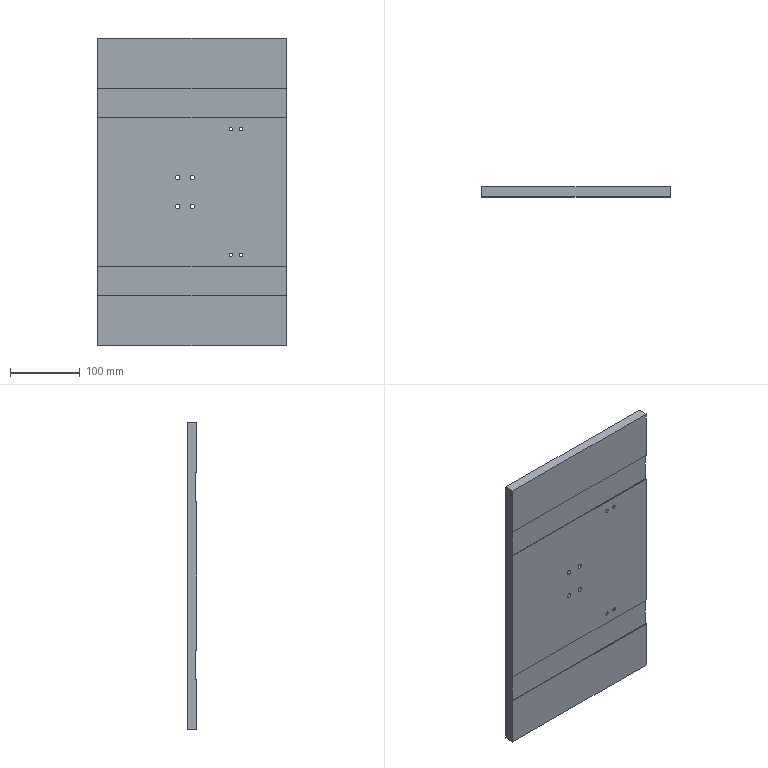Part | SolidWorks | features ICE 3, 3DProfileFeature 1, Extrusion 1, HoleWzd 1 | 1 solid | 47 faces | box 270 x 14 x 440 mm | volume 1620625 mm3 | cylinder 24 | plane 23 | commonest cylinder face diameters 5 x8 6.6 x8 11 x8
STEP:
#1=CARTESIAN_POINT('',(70.,0.,-92.5));
#2=VERTEX_POINT('',#1);
#3=CARTESIAN_POINT('',(70.,0.,-87.5));
#4=VERTEX_POINT('',#3);
#5=CARTESIAN_POINT('',(70.,0.,-90.));
#6=DIRECTION('',(0.,1.,0.));
#7=DIRECTION('',(0.,0.,-1.));
#8=AXIS2_PLACEMENT_3D('',#5,#6,#7);
#9=CIRCLE('',#8,2.5);
#10=EDGE_CURVE('',#2,#4,#9,.T.);
#11=ORIENTED_EDGE('',*,*,#10,.F.);
#12=CARTESIAN_POINT('',(70.,14.,-92.5));
#13=VERTEX_POINT('',#12);
#14=CARTESIAN_POINT('',(70.,-0.001,-92.5));
#15=DIRECTION('',(0.,1.,0.));
#16=VECTOR('',#15,1000.);
#17=LINE('',#14,#16);
#18=EDGE_CURVE('',#2,#13,#17,.T.);
#19=ORIENTED_EDGE('',*,*,#18,.T.);
#20=CARTESIAN_POINT('',(67.5,14.,-90.));
#21=VERTEX_POINT('',#20);
#22=CARTESIAN_POINT('',(70.,14.,-90.));
#23=DIRECTION('',(0.,1.,0.));
#24=DIRECTION('',(0.,0.,1.));
#25=AXIS2_PLACEMENT_3D('',#22,#23,#24);
#26=CIRCLE('',#25,2.5);
#27=EDGE_CURVE('',#13,#21,#26,.T.);
#28=ORIENTED_EDGE('',*,*,#27,.T.);
#29=CARTESIAN_POINT('',(67.5,12.5,-90.));
#30=VERTEX_POINT('',#29);
#31=CARTESIAN_POINT('',(67.5,-0.001,-90.));
#32=DIRECTION('',(0.,-1.,0.));
#33=VECTOR('',#32,1000.);
#34=LINE('',#31,#33);
#35=EDGE_CURVE('',#21,#30,#34,.T.);
#36=ORIENTED_EDGE('',*,*,#35,.T.);
#37=CARTESIAN_POINT('',(70.,12.5,-87.5));
#38=VERTEX_POINT('',#37);
#39=CARTESIAN_POINT('',(70.,12.5,-90.));
#40=DIRECTION('',(0.,-1.,0.));
#41=DIRECTION('',(0.,0.,1.));
#42=AXIS2_PLACEMENT_3D('',#39,#40,#41);
#43=CIRCLE('',#42,2.5);
#44=EDGE_CURVE('',#38,#30,#43,.T.);
#45=ORIENTED_EDGE('',*,*,#44,.F.);
#46=CARTESIAN_POINT('',(70.,-0.001,-87.5));
#47=DIRECTION('',(0.,1.,0.));
#48=VECTOR('',#47,1000.);
#49=LINE('',#46,#48);
#50=EDGE_CURVE('',#4,#38,#49,.T.);
#51=ORIENTED_EDGE('',*,*,#50,.F.);
#52=EDGE_LOOP('',(#11,#19,#28,#36,#45,#51));
#53=FACE_OUTER_BOUND('',#52,.T.);
#54=CARTESIAN_POINT('',(70.,-0.001,-90.));
#55=DIRECTION('',(0.,1.,0.));
#56=DIRECTION('',(0.,0.,1.));
#57=AXIS2_PLACEMENT_3D('',#54,#55,#56);
#58=CYLINDRICAL_SURFACE('',#57,2.5);
#59=ADVANCED_FACE('',(#53),#58,.F.);
#60=CARTESIAN_POINT('',(55.5,0.,87.5));
#61=VERTEX_POINT('',#60);
#62=CARTESIAN_POINT('',(55.5,0.,92.5));
#63=VERTEX_POINT('',#62);
#64=CARTESIAN_POINT('',(55.5,0.,90.));
#65=DIRECTION('',(0.,1.,0.));
#66=DIRECTION('',(0.,0.,-1.));
#67=AXIS2_PLACEMENT_3D('',#64,#65,#66);
#68=CIRCLE('',#67,2.5);
#69=EDGE_CURVE('',#61,#63,#68,.T.);
#70=ORIENTED_EDGE('',*,*,#69,.F.);
#71=CARTESIAN_POINT('',(55.5,12.5,87.5));
#72=VERTEX_POINT('',#71);
#73=CARTESIAN_POINT('',(55.5,-0.001,87.5));
#74=DIRECTION('',(0.,1.,0.));
#75=VECTOR('',#74,1000.);
#76=LINE('',#73,#75);
#77=EDGE_CURVE('',#61,#72,#76,.T.);
#78=ORIENTED_EDGE('',*,*,#77,.T.);
#79=CARTESIAN_POINT('',(55.5,14.,87.5));
#80=VERTEX_POINT('',#79);
#81=CARTESIAN_POINT('',(55.5,-0.001,87.5));
#82=DIRECTION('',(0.,1.,0.));
#83=VECTOR('',#82,1000.);
#84=LINE('',#81,#83);
#85=EDGE_CURVE('',#72,#80,#84,.T.);
#86=ORIENTED_EDGE('',*,*,#85,.T.);
#87=CARTESIAN_POINT('',(55.5,14.,92.5));
#88=VERTEX_POINT('',#87);
#89=CARTESIAN_POINT('',(55.5,14.,90.));
#90=DIRECTION('',(0.,1.,0.));
#91=DIRECTION('',(0.,0.,1.));
#92=AXIS2_PLACEMENT_3D('',#89,#90,#91);
#93=CIRCLE('',#92,2.5);
#94=EDGE_CURVE('',#80,#88,#93,.T.);
#95=ORIENTED_EDGE('',*,*,#94,.T.);
#96=CARTESIAN_POINT('',(55.5,-0.001,92.5));
#97=DIRECTION('',(0.,1.,0.));
#98=VECTOR('',#97,1000.);
#99=LINE('',#96,#98);
#100=EDGE_CURVE('',#63,#88,#99,.T.);
#101=ORIENTED_EDGE('',*,*,#100,.F.);
#102=EDGE_LOOP('',(#70,#78,#86,#95,#101));
#103=FACE_OUTER_BOUND('',#102,.T.);
#104=CARTESIAN_POINT('',(55.5,-0.001,90.));
#105=DIRECTION('',(0.,1.,0.));
#106=DIRECTION('',(0.,0.,1.));
#107=AXIS2_PLACEMENT_3D('',#104,#105,#106);
#108=CYLINDRICAL_SURFACE('',#107,2.5);
#109=ADVANCED_FACE('',(#103),#108,.F.);
#110=CARTESIAN_POINT('',(70.,0.,87.5));
#111=VERTEX_POINT('',#110);
#112=CARTESIAN_POINT('',(70.,0.,92.5));
#113=VERTEX_POINT('',#112);
#114=CARTESIAN_POINT('',(70.,0.,90.));
#115=DIRECTION('',(0.,1.,0.));
#116=DIRECTION('',(0.,0.,-1.));
#117=AXIS2_PLACEMENT_3D('',#114,#115,#116);
#118=CIRCLE('',#117,2.5);
#119=EDGE_CURVE('',#111,#113,#118,.T.);
#120=ORIENTED_EDGE('',*,*,#119,.F.);
#121=CARTESIAN_POINT('',(70.,12.5,87.5));
#122=VERTEX_POINT('',#121);
#123=CARTESIAN_POINT('',(70.,-0.001,87.5));
#124=DIRECTION('',(0.,1.,0.));
#125=VECTOR('',#124,1000.);
#126=LINE('',#123,#125);
#127=EDGE_CURVE('',#111,#122,#126,.T.);
#128=ORIENTED_EDGE('',*,*,#127,.T.);
#129=CARTESIAN_POINT('',(67.5,12.5,90.));
#130=VERTEX_POINT('',#129);
#131=CARTESIAN_POINT('',(70.,12.5,90.));
#132=DIRECTION('',(0.,-1.,0.));
#133=DIRECTION('',(0.,0.,1.));
#134=AXIS2_PLACEMENT_3D('',#131,#132,#133);
#135=CIRCLE('',#134,2.5);
#136=EDGE_CURVE('',#130,#122,#135,.T.);
#137=ORIENTED_EDGE('',*,*,#136,.F.);
#138=CARTESIAN_POINT('',(67.5,14.,90.));
#139=VERTEX_POINT('',#138);
#140=CARTESIAN_POINT('',(67.5,-0.001,90.));
#141=DIRECTION('',(0.,1.,0.));
#142=VECTOR('',#141,1000.);
#143=LINE('',#140,#142);
#144=EDGE_CURVE('',#130,#139,#143,.T.);
#145=ORIENTED_EDGE('',*,*,#144,.T.);
#146=CARTESIAN_POINT('',(70.,14.,92.5));
#147=VERTEX_POINT('',#146);
#148=CARTESIAN_POINT('',(70.,14.,90.));
#149=DIRECTION('',(0.,1.,0.));
#150=DIRECTION('',(0.,0.,1.));
#151=AXIS2_PLACEMENT_3D('',#148,#149,#150);
#152=CIRCLE('',#151,2.5);
#153=EDGE_CURVE('',#139,#147,#152,.T.);
#154=ORIENTED_EDGE('',*,*,#153,.T.);
#155=CARTESIAN_POINT('',(70.,-0.001,92.5));
#156=DIRECTION('',(0.,1.,0.));
#157=VECTOR('',#156,1000.);
#158=LINE('',#155,#157);
#159=EDGE_CURVE('',#113,#147,#158,.T.);
#160=ORIENTED_EDGE('',*,*,#159,.F.);
#161=EDGE_LOOP('',(#120,#128,#137,#145,#154,#160));
#162=FACE_OUTER_BOUND('',#161,.T.);
#163=CARTESIAN_POINT('',(70.,-0.001,90.));
#164=DIRECTION('',(0.,1.,0.));
#165=DIRECTION('',(0.,0.,1.));
#166=AXIS2_PLACEMENT_3D('',#163,#164,#165);
#167=CYLINDRICAL_SURFACE('',#166,2.5);
#168=ADVANCED_FACE('',(#162),#167,.F.);
#169=CARTESIAN_POINT('',(55.5,0.,-92.5));
#170=VERTEX_POINT('',#169);
#171=CARTESIAN_POINT('',(55.5,0.,-87.5));
#172=VERTEX_POINT('',#171);
#173=CARTESIAN_POINT('',(55.5,0.,-90.));
#174=DIRECTION('',(0.,1.,0.));
#175=DIRECTION('',(0.,0.,-1.));
#176=AXIS2_PLACEMENT_3D('',#173,#174,#175);
#177=CIRCLE('',#176,2.5);
#178=EDGE_CURVE('',#170,#172,#177,.T.);
#179=ORIENTED_EDGE('',*,*,#178,.F.);
#180=CARTESIAN_POINT('',(55.5,14.,-92.5));
#181=VERTEX_POINT('',#180);
#182=CARTESIAN_POINT('',(55.5,-0.001,-92.5));
#183=DIRECTION('',(0.,1.,0.));
#184=VECTOR('',#183,1000.);
#185=LINE('',#182,#184);
#186=EDGE_CURVE('',#170,#181,#185,.T.);
#187=ORIENTED_EDGE('',*,*,#186,.T.);
#188=CARTESIAN_POINT('',(55.5,14.,-87.5));
#189=VERTEX_POINT('',#188);
#190=CARTESIAN_POINT('',(55.5,14.,-90.));
#191=DIRECTION('',(0.,1.,0.));
#192=DIRECTION('',(0.,0.,1.));
#193=AXIS2_PLACEMENT_3D('',#190,#191,#192);
#194=CIRCLE('',#193,2.5);
#195=EDGE_CURVE('',#181,#189,#194,.T.);
#196=ORIENTED_EDGE('',*,*,#195,.T.);
#197=CARTESIAN_POINT('',(55.5,12.5,-87.5));
#198=VERTEX_POINT('',#197);
#199=CARTESIAN_POINT('',(55.5,-0.001,-87.5));
#200=DIRECTION('',(0.,-1.,0.));
#201=VECTOR('',#200,1000.);
#202=LINE('',#199,#201);
#203=EDGE_CURVE('',#189,#198,#202,.T.);
#204=ORIENTED_EDGE('',*,*,#203,.T.);
#205=CARTESIAN_POINT('',(55.5,-0.001,-87.5));
#206=DIRECTION('',(0.,1.,0.));
#207=VECTOR('',#206,1000.);
#208=LINE('',#205,#207);
#209=EDGE_CURVE('',#172,#198,#208,.T.);
#210=ORIENTED_EDGE('',*,*,#209,.F.);
#211=EDGE_LOOP('',(#179,#187,#196,#204,#210));
#212=FACE_OUTER_BOUND('',#211,.T.);
#213=CARTESIAN_POINT('',(55.5,-0.001,-90.));
#214=DIRECTION('',(0.,1.,0.));
#215=DIRECTION('',(0.,0.,1.));
#216=AXIS2_PLACEMENT_3D('',#213,#214,#215);
#217=CYLINDRICAL_SURFACE('',#216,2.5);
#218=ADVANCED_FACE('',(#212),#217,.F.);
#219=CARTESIAN_POINT('',(-20.55,7.2,15.));
#220=VERTEX_POINT('',#219);
#221=CARTESIAN_POINT('',(-20.55,7.2,26.));
#222=VERTEX_POINT('',#221);
#223=CARTESIAN_POINT('',(-20.55,7.2,20.5));
#224=DIRECTION('',(0.,1.,0.));
#225=DIRECTION('',(0.,0.,1.));
#226=AXIS2_PLACEMENT_3D('',#223,#224,#225);
#227=CIRCLE('',#226,5.5);
#228=EDGE_CURVE('',#220,#222,#227,.T.);
#229=ORIENTED_EDGE('',*,*,#228,.F.);
#230=CARTESIAN_POINT('',(-20.55,14.,15.));
#231=VERTEX_POINT('',#230);
#232=CARTESIAN_POINT('',(-20.55,14.,15.));
#233=DIRECTION('',(0.,1.,0.));
#234=VECTOR('',#233,1000.);
#235=LINE('',#232,#234);
#236=EDGE_CURVE('',#220,#231,#235,.T.);
#237=ORIENTED_EDGE('',*,*,#236,.T.);
#238=CARTESIAN_POINT('',(-20.55,14.,26.));
#239=VERTEX_POINT('',#238);
#240=CARTESIAN_POINT('',(-20.55,14.,20.5));
#241=DIRECTION('',(0.,1.,0.));
#242=DIRECTION('',(0.,0.,1.));
#243=AXIS2_PLACEMENT_3D('',#240,#241,#242);
#244=CIRCLE('',#243,5.5);
#245=EDGE_CURVE('',#231,#239,#244,.T.);
#246=ORIENTED_EDGE('',*,*,#245,.T.);
#247=CARTESIAN_POINT('',(-20.55,14.,26.));
#248=DIRECTION('',(0.,1.,0.));
#249=VECTOR('',#248,1000.);
#250=LINE('',#247,#249);
#251=EDGE_CURVE('',#222,#239,#250,.T.);
#252=ORIENTED_EDGE('',*,*,#251,.F.);
#253=EDGE_LOOP('',(#229,#237,#246,#252));
#254=FACE_OUTER_BOUND('',#253,.T.);
#255=CARTESIAN_POINT('',(-20.55,14.,20.5));
#256=DIRECTION('',(0.,1.,0.));
#257=DIRECTION('',(0.,0.,1.));
#258=AXIS2_PLACEMENT_3D('',#255,#256,#257);
#259=CYLINDRICAL_SURFACE('',#258,5.5);
#260=ADVANCED_FACE('',(#254),#259,.F.);
#261=CARTESIAN_POINT('',(-20.55,0.,23.8));
#262=VERTEX_POINT('',#261);
#263=CARTESIAN_POINT('',(-20.55,0.,17.2));
#264=VERTEX_POINT('',#263);
#265=CARTESIAN_POINT('',(-20.55,0.,20.5));
#266=DIRECTION('',(0.,-1.,0.));
#267=DIRECTION('',(0.,0.,-1.));
#268=AXIS2_PLACEMENT_3D('',#265,#266,#267);
#269=CIRCLE('',#268,3.3);
#270=EDGE_CURVE('',#262,#264,#269,.T.);
#271=ORIENTED_EDGE('',*,*,#270,.T.);
#272=CARTESIAN_POINT('',(-20.55,7.2,17.2));
#273=VERTEX_POINT('',#272);
#274=CARTESIAN_POINT('',(-20.55,14.,17.2));
#275=DIRECTION('',(0.,1.,0.));
#276=VECTOR('',#275,1000.);
#277=LINE('',#274,#276);
#278=EDGE_CURVE('',#264,#273,#277,.T.);
#279=ORIENTED_EDGE('',*,*,#278,.T.);
#280=CARTESIAN_POINT('',(-20.55,7.2,23.8));
#281=VERTEX_POINT('',#280);
#282=CARTESIAN_POINT('',(-20.55,7.2,20.5));
#283=DIRECTION('',(0.,1.,0.));
#284=DIRECTION('',(0.,0.,1.));
#285=AXIS2_PLACEMENT_3D('',#282,#283,#284);
#286=CIRCLE('',#285,3.3);
#287=EDGE_CURVE('',#273,#281,#286,.T.);
#288=ORIENTED_EDGE('',*,*,#287,.T.);
#289=CARTESIAN_POINT('',(-20.55,14.,23.8));
#290=DIRECTION('',(0.,1.,0.));
#291=VECTOR('',#290,1000.);
#292=LINE('',#289,#291);
#293=EDGE_CURVE('',#262,#281,#292,.T.);
#294=ORIENTED_EDGE('',*,*,#293,.F.);
#295=EDGE_LOOP('',(#271,#279,#288,#294));
#296=FACE_OUTER_BOUND('',#295,.T.);
#297=CARTESIAN_POINT('',(-20.55,14.,20.5));
#298=DIRECTION('',(0.,1.,0.));
#299=DIRECTION('',(0.,0.,1.));
#300=AXIS2_PLACEMENT_3D('',#297,#298,#299);
#301=CYLINDRICAL_SURFACE('',#300,3.3);
#302=ADVANCED_FACE('',(#296),#301,.F.);
#303=CARTESIAN_POINT('',(-20.55,7.2,-26.));
#304=VERTEX_POINT('',#303);
#305=CARTESIAN_POINT('',(-20.55,7.2,-15.));
#306=VERTEX_POINT('',#305);
#307=CARTESIAN_POINT('',(-20.55,7.2,-20.5));
#308=DIRECTION('',(0.,1.,0.));
#309=DIRECTION('',(0.,0.,1.));
#310=AXIS2_PLACEMENT_3D('',#307,#308,#309);
#311=CIRCLE('',#310,5.5);
#312=EDGE_CURVE('',#304,#306,#311,.T.);
#313=ORIENTED_EDGE('',*,*,#312,.F.);
#314=CARTESIAN_POINT('',(-20.55,14.,-26.));
#315=VERTEX_POINT('',#314);
#316=CARTESIAN_POINT('',(-20.55,14.,-26.));
#317=DIRECTION('',(0.,1.,0.));
#318=VECTOR('',#317,1000.);
#319=LINE('',#316,#318);
#320=EDGE_CURVE('',#304,#315,#319,.T.);
#321=ORIENTED_EDGE('',*,*,#320,.T.);
#322=CARTESIAN_POINT('',(-20.55,14.,-15.));
#323=VERTEX_POINT('',#322);
#324=CARTESIAN_POINT('',(-20.55,14.,-20.5));
#325=DIRECTION('',(0.,1.,0.));
#326=DIRECTION('',(0.,0.,1.));
#327=AXIS2_PLACEMENT_3D('',#324,#325,#326);
#328=CIRCLE('',#327,5.5);
#329=EDGE_CURVE('',#315,#323,#328,.T.);
#330=ORIENTED_EDGE('',*,*,#329,.T.);
#331=CARTESIAN_POINT('',(-20.55,14.,-15.));
#332=DIRECTION('',(0.,1.,0.));
#333=VECTOR('',#332,1000.);
#334=LINE('',#331,#333);
#335=EDGE_CURVE('',#306,#323,#334,.T.);
#336=ORIENTED_EDGE('',*,*,#335,.F.);
#337=EDGE_LOOP('',(#313,#321,#330,#336));
#338=FACE_OUTER_BOUND('',#337,.T.);
#339=CARTESIAN_POINT('',(-20.55,14.,-20.5));
#340=DIRECTION('',(0.,1.,0.));
#341=DIRECTION('',(0.,0.,1.));
#342=AXIS2_PLACEMENT_3D('',#339,#340,#341);
#343=CYLINDRICAL_SURFACE('',#342,5.5);
#344=ADVANCED_FACE('',(#338),#343,.F.);
#345=CARTESIAN_POINT('',(-20.55,0.,-17.2));
#346=VERTEX_POINT('',#345);
#347=CARTESIAN_POINT('',(-20.55,0.,-23.8));
#348=VERTEX_POINT('',#347);
#349=CARTESIAN_POINT('',(-20.55,0.,-20.5));
#350=DIRECTION('',(0.,-1.,0.));
#351=DIRECTION('',(0.,0.,-1.));
#352=AXIS2_PLACEMENT_3D('',#349,#350,#351);
#353=CIRCLE('',#352,3.3);
#354=EDGE_CURVE('',#346,#348,#353,.T.);
#355=ORIENTED_EDGE('',*,*,#354,.T.);
#356=CARTESIAN_POINT('',(-20.55,7.2,-23.8));
#357=VERTEX_POINT('',#356);
#358=CARTESIAN_POINT('',(-20.55,14.,-23.8));
#359=DIRECTION('',(0.,1.,0.));
#360=VECTOR('',#359,1000.);
#361=LINE('',#358,#360);
#362=EDGE_CURVE('',#348,#357,#361,.T.);
#363=ORIENTED_EDGE('',*,*,#362,.T.);
#364=CARTESIAN_POINT('',(-20.55,7.2,-17.2));
#365=VERTEX_POINT('',#364);
#366=CARTESIAN_POINT('',(-20.55,7.2,-20.5));
#367=DIRECTION('',(0.,1.,0.));
#368=DIRECTION('',(0.,0.,1.));
#369=AXIS2_PLACEMENT_3D('',#366,#367,#368);
#370=CIRCLE('',#369,3.3);
#371=EDGE_CURVE('',#357,#365,#370,.T.);
#372=ORIENTED_EDGE('',*,*,#371,.T.);
#373=CARTESIAN_POINT('',(-20.55,14.,-17.2));
#374=DIRECTION('',(0.,1.,0.));
#375=VECTOR('',#374,1000.);
#376=LINE('',#373,#375);
#377=EDGE_CURVE('',#346,#365,#376,.T.);
#378=ORIENTED_EDGE('',*,*,#377,.F.);
#379=EDGE_LOOP('',(#355,#363,#372,#378));
#380=FACE_OUTER_BOUND('',#379,.T.);
#381=CARTESIAN_POINT('',(-20.55,14.,-20.5));
#382=DIRECTION('',(0.,1.,0.));
#383=DIRECTION('',(0.,0.,1.));
#384=AXIS2_PLACEMENT_3D('',#381,#382,#383);
#385=CYLINDRICAL_SURFACE('',#384,3.3);
#386=ADVANCED_FACE('',(#380),#385,.F.);
#387=CARTESIAN_POINT('',(0.45,7.2,15.));
#388=VERTEX_POINT('',#387);
#389=CARTESIAN_POINT('',(0.45,7.2,26.));
#390=VERTEX_POINT('',#389);
#391=CARTESIAN_POINT('',(0.45,7.2,20.5));
#392=DIRECTION('',(0.,1.,0.));
#393=DIRECTION('',(0.,0.,1.));
#394=AXIS2_PLACEMENT_3D('',#391,#392,#393);
#395=CIRCLE('',#394,5.5);
#396=EDGE_CURVE('',#388,#390,#395,.T.);
#397=ORIENTED_EDGE('',*,*,#396,.F.);
#398=CARTESIAN_POINT('',(0.45,14.,15.));
#399=VERTEX_POINT('',#398);
#400=CARTESIAN_POINT('',(0.45,14.,15.));
#401=DIRECTION('',(0.,1.,0.));
#402=VECTOR('',#401,1000.);
#403=LINE('',#400,#402);
#404=EDGE_CURVE('',#388,#399,#403,.T.);
#405=ORIENTED_EDGE('',*,*,#404,.T.);
#406=CARTESIAN_POINT('',(0.45,14.,26.));
#407=VERTEX_POINT('',#406);
#408=CARTESIAN_POINT('',(0.45,14.,20.5));
#409=DIRECTION('',(0.,1.,0.));
#410=DIRECTION('',(0.,0.,1.));
#411=AXIS2_PLACEMENT_3D('',#408,#409,#410);
#412=CIRCLE('',#411,5.5);
#413=EDGE_CURVE('',#399,#407,#412,.T.);
#414=ORIENTED_EDGE('',*,*,#413,.T.);
#415=CARTESIAN_POINT('',(0.45,14.,26.));
#416=DIRECTION('',(0.,1.,0.));
#417=VECTOR('',#416,1000.);
#418=LINE('',#415,#417);
#419=EDGE_CURVE('',#390,#407,#418,.T.);
#420=ORIENTED_EDGE('',*,*,#419,.F.);
#421=EDGE_LOOP('',(#397,#405,#414,#420));
#422=FACE_OUTER_BOUND('',#421,.T.);
#423=CARTESIAN_POINT('',(0.45,14.,20.5));
#424=DIRECTION('',(0.,1.,0.));
#425=DIRECTION('',(0.,0.,1.));
#426=AXIS2_PLACEMENT_3D('',#423,#424,#425);
#427=CYLINDRICAL_SURFACE('',#426,5.5);
#428=ADVANCED_FACE('',(#422),#427,.F.);
#429=CARTESIAN_POINT('',(0.45,0.,23.8));
#430=VERTEX_POINT('',#429);
#431=CARTESIAN_POINT('',(0.45,0.,17.2));
#432=VERTEX_POINT('',#431);
#433=CARTESIAN_POINT('',(0.45,0.,20.5));
#434=DIRECTION('',(0.,-1.,0.));
#435=DIRECTION('',(0.,0.,-1.));
#436=AXIS2_PLACEMENT_3D('',#433,#434,#435);
#437=CIRCLE('',#436,3.3);
#438=EDGE_CURVE('',#430,#432,#437,.T.);
#439=ORIENTED_EDGE('',*,*,#438,.T.);
#440=CARTESIAN_POINT('',(0.45,7.2,17.2));
#441=VERTEX_POINT('',#440);
#442=CARTESIAN_POINT('',(0.45,14.,17.2));
#443=DIRECTION('',(0.,1.,0.));
#444=VECTOR('',#443,1000.);
#445=LINE('',#442,#444);
#446=EDGE_CURVE('',#432,#441,#445,.T.);
#447=ORIENTED_EDGE('',*,*,#446,.T.);
#448=CARTESIAN_POINT('',(0.45,7.2,23.8));
#449=VERTEX_POINT('',#448);
#450=CARTESIAN_POINT('',(0.45,7.2,20.5));
#451=DIRECTION('',(0.,1.,0.));
#452=DIRECTION('',(0.,0.,1.));
#453=AXIS2_PLACEMENT_3D('',#450,#451,#452);
#454=CIRCLE('',#453,3.3);
#455=EDGE_CURVE('',#441,#449,#454,.T.);
#456=ORIENTED_EDGE('',*,*,#455,.T.);
#457=CARTESIAN_POINT('',(0.45,14.,23.8));
#458=DIRECTION('',(0.,1.,0.));
#459=VECTOR('',#458,1000.);
#460=LINE('',#457,#459);
#461=EDGE_CURVE('',#430,#449,#460,.T.);
#462=ORIENTED_EDGE('',*,*,#461,.F.);
#463=EDGE_LOOP('',(#439,#447,#456,#462));
#464=FACE_OUTER_BOUND('',#463,.T.);
#465=CARTESIAN_POINT('',(0.45,14.,20.5));
#466=DIRECTION('',(0.,1.,0.));
#467=DIRECTION('',(0.,0.,1.));
#468=AXIS2_PLACEMENT_3D('',#465,#466,#467);
#469=CYLINDRICAL_SURFACE('',#468,3.3);
#470=ADVANCED_FACE('',(#464),#469,.F.);
#471=CARTESIAN_POINT('',(0.45,7.2,-26.));
#472=VERTEX_POINT('',#471);
#473=CARTESIAN_POINT('',(0.45,7.2,-15.));
#474=VERTEX_POINT('',#473);
#475=CARTESIAN_POINT('',(0.45,7.2,-20.5));
#476=DIRECTION('',(0.,1.,0.));
#477=DIRECTION('',(0.,0.,1.));
#478=AXIS2_PLACEMENT_3D('',#475,#476,#477);
#479=CIRCLE('',#478,5.5);
#480=EDGE_CURVE('',#472,#474,#479,.T.);
#481=ORIENTED_EDGE('',*,*,#480,.F.);
#482=CARTESIAN_POINT('',(0.45,14.,-26.));
#483=VERTEX_POINT('',#482);
#484=CARTESIAN_POINT('',(0.45,14.,-26.));
#485=DIRECTION('',(0.,1.,0.));
#486=VECTOR('',#485,1000.);
#487=LINE('',#484,#486);
#488=EDGE_CURVE('',#472,#483,#487,.T.);
#489=ORIENTED_EDGE('',*,*,#488,.T.);
#490=CARTESIAN_POINT('',(0.45,14.,-15.));
#491=VERTEX_POINT('',#490);
#492=CARTESIAN_POINT('',(0.45,14.,-20.5));
#493=DIRECTION('',(0.,1.,0.));
#494=DIRECTION('',(0.,0.,1.));
#495=AXIS2_PLACEMENT_3D('',#492,#493,#494);
#496=CIRCLE('',#495,5.5);
#497=EDGE_CURVE('',#483,#491,#496,.T.);
#498=ORIENTED_EDGE('',*,*,#497,.T.);
#499=CARTESIAN_POINT('',(0.45,14.,-15.));
#500=DIRECTION('',(0.,1.,0.));
#501=VECTOR('',#500,1000.);
#502=LINE('',#499,#501);
#503=EDGE_CURVE('',#474,#491,#502,.T.);
#504=ORIENTED_EDGE('',*,*,#503,.F.);
#505=EDGE_LOOP('',(#481,#489,#498,#504));
#506=FACE_OUTER_BOUND('',#505,.T.);
#507=CARTESIAN_POINT('',(0.45,14.,-20.5));
#508=DIRECTION('',(0.,1.,0.));
#509=DIRECTION('',(0.,0.,1.));
#510=AXIS2_PLACEMENT_3D('',#507,#508,#509);
#511=CYLINDRICAL_SURFACE('',#510,5.5);
#512=ADVANCED_FACE('',(#506),#511,.F.);
#513=CARTESIAN_POINT('',(0.45,0.,-17.2));
#514=VERTEX_POINT('',#513);
#515=CARTESIAN_POINT('',(0.45,0.,-23.8));
#516=VERTEX_POINT('',#515);
#517=CARTESIAN_POINT('',(0.45,0.,-20.5));
#518=DIRECTION('',(0.,-1.,0.));
#519=DIRECTION('',(0.,0.,-1.));
#520=AXIS2_PLACEMENT_3D('',#517,#518,#519);
#521=CIRCLE('',#520,3.3);
#522=EDGE_CURVE('',#514,#516,#521,.T.);
#523=ORIENTED_EDGE('',*,*,#522,.T.);
#524=CARTESIAN_POINT('',(0.45,7.2,-23.8));
#525=VERTEX_POINT('',#524);
#526=CARTESIAN_POINT('',(0.45,14.,-23.8));
#527=DIRECTION('',(0.,1.,0.));
#528=VECTOR('',#527,1000.);
#529=LINE('',#526,#528);
#530=EDGE_CURVE('',#516,#525,#529,.T.);
#531=ORIENTED_EDGE('',*,*,#530,.T.);
#532=CARTESIAN_POINT('',(0.45,7.2,-17.2));
#533=VERTEX_POINT('',#532);
#534=CARTESIAN_POINT('',(0.45,7.2,-20.5));
#535=DIRECTION('',(0.,1.,0.));
#536=DIRECTION('',(0.,0.,1.));
#537=AXIS2_PLACEMENT_3D('',#534,#535,#536);
#538=CIRCLE('',#537,3.3);
#539=EDGE_CURVE('',#525,#533,#538,.T.);
#540=ORIENTED_EDGE('',*,*,#539,.T.);
#541=CARTESIAN_POINT('',(0.45,14.,-17.2));
#542=DIRECTION('',(0.,1.,0.));
#543=VECTOR('',#542,1000.);
#544=LINE('',#541,#543);
#545=EDGE_CURVE('',#514,#533,#544,.T.);
#546=ORIENTED_EDGE('',*,*,#545,.F.);
#547=EDGE_LOOP('',(#523,#531,#540,#546));
#548=FACE_OUTER_BOUND('',#547,.T.);
#549=CARTESIAN_POINT('',(0.45,14.,-20.5));
#550=DIRECTION('',(0.,1.,0.));
#551=DIRECTION('',(0.,0.,1.));
#552=AXIS2_PLACEMENT_3D('',#549,#550,#551);
#553=CYLINDRICAL_SURFACE('',#552,3.3);
#554=ADVANCED_FACE('',(#548),#553,.F.);
#555=CARTESIAN_POINT('',(135.,0.,148.));
#556=VERTEX_POINT('',#555);
#557=CARTESIAN_POINT('',(-135.,0.,148.));
#558=VERTEX_POINT('',#557);
#559=CARTESIAN_POINT('',(-135.,0.,148.));
#560=DIRECTION('',(-1.,0.,0.));
#561=VECTOR('',#560,1000.);
#562=LINE('',#559,#561);
#563=EDGE_CURVE('',#556,#558,#562,.T.);
#564=ORIENTED_EDGE('',*,*,#563,.F.);
#565=CARTESIAN_POINT('',(135.,0.,220.));
#566=VERTEX_POINT('',#565);
#567=CARTESIAN_POINT('',(135.,0.,220.));
#568=DIRECTION('',(0.,0.,-1.));
#569=VECTOR('',#568,1000.);
#570=LINE('',#567,#569);
#571=EDGE_CURVE('',#566,#556,#570,.T.);
#572=ORIENTED_EDGE('',*,*,#571,.F.);
#573=CARTESIAN_POINT('',(-135.,0.,220.));
#574=VERTEX_POINT('',#573);
#575=CARTESIAN_POINT('',(-135.,0.,220.));
#576=DIRECTION('',(1.,0.,0.));
#577=VECTOR('',#576,1000.);
#578=LINE('',#575,#577);
#579=EDGE_CURVE('',#574,#566,#578,.T.);
#580=ORIENTED_EDGE('',*,*,#579,.F.);
#581=CARTESIAN_POINT('',(-135.,0.,220.));
#582=DIRECTION('',(0.,0.,1.));
#583=VECTOR('',#582,1000.);
#584=LINE('',#581,#583);
#585=EDGE_CURVE('',#558,#574,#584,.T.);
#586=ORIENTED_EDGE('',*,*,#585,.F.);
#587=EDGE_LOOP('',(#564,#572,#580,#586));
#588=FACE_OUTER_BOUND('',#587,.T.);
#589=CARTESIAN_POINT('',(0.,0.,0.));
#590=DIRECTION('',(0.,-1.,0.));
#591=DIRECTION('',(0.,0.,-1.));
#592=AXIS2_PLACEMENT_3D('',#589,#590,#591);
#593=PLANE('',#592);
#594=ADVANCED_FACE('',(#588),#593,.T.);
#595=CARTESIAN_POINT('',(70.,0.,-90.));
#596=DIRECTION('',(0.,1.,0.));
#597=DIRECTION('',(0.,0.,-1.));
#598=AXIS2_PLACEMENT_3D('',#595,#596,#597);
#599=CIRCLE('',#598,2.5);
#600=EDGE_CURVE('',#4,#2,#599,.T.);
#601=ORIENTED_EDGE('',*,*,#600,.T.);
#602=ORIENTED_EDGE('',*,*,#10,.T.);
#603=EDGE_LOOP('',(#601,#602));
#604=FACE_BOUND('',#603,.T.);
#605=CARTESIAN_POINT('',(55.5,0.,90.));
#606=DIRECTION('',(0.,1.,0.));
#607=DIRECTION('',(0.,0.,-1.));
#608=AXIS2_PLACEMENT_3D('',#605,#606,#607);
#609=CIRCLE('',#608,2.5);
#610=EDGE_CURVE('',#63,#61,#609,.T.);
#611=ORIENTED_EDGE('',*,*,#610,.T.);
#612=ORIENTED_EDGE('',*,*,#69,.T.);
#613=EDGE_LOOP('',(#611,#612));
#614=FACE_BOUND('',#613,.T.);
#615=CARTESIAN_POINT('',(70.,0.,90.));
#616=DIRECTION('',(0.,1.,0.));
#617=DIRECTION('',(0.,0.,-1.));
#618=AXIS2_PLACEMENT_3D('',#615,#616,#617);
#619=CIRCLE('',#618,2.5);
#620=EDGE_CURVE('',#113,#111,#619,.T.);
#621=ORIENTED_EDGE('',*,*,#620,.T.);
#622=ORIENTED_EDGE('',*,*,#119,.T.);
#623=EDGE_LOOP('',(#621,#622));
#624=FACE_BOUND('',#623,.T.);
#625=CARTESIAN_POINT('',(55.5,0.,-90.));
#626=DIRECTION('',(0.,1.,0.));
#627=DIRECTION('',(0.,0.,-1.));
#628=AXIS2_PLACEMENT_3D('',#625,#626,#627);
#629=CIRCLE('',#628,2.5);
#630=EDGE_CURVE('',#172,#170,#629,.T.);
#631=ORIENTED_EDGE('',*,*,#630,.T.);
#632=ORIENTED_EDGE('',*,*,#178,.T.);
#633=EDGE_LOOP('',(#631,#632));
#634=FACE_BOUND('',#633,.T.);
#635=ORIENTED_EDGE('',*,*,#270,.F.);
#636=CARTESIAN_POINT('',(-20.55,0.,20.5));
#637=DIRECTION('',(0.,-1.,0.));
#638=DIRECTION('',(0.,0.,-1.));
#639=AXIS2_PLACEMENT_3D('',#636,#637,#638);
#640=CIRCLE('',#639,3.3);
#641=EDGE_CURVE('',#264,#262,#640,.T.);
#642=ORIENTED_EDGE('',*,*,#641,.F.);
#643=EDGE_LOOP('',(#635,#642));
#644=FACE_BOUND('',#643,.T.);
#645=ORIENTED_EDGE('',*,*,#354,.F.);
#646=CARTESIAN_POINT('',(-20.55,0.,-20.5));
#647=DIRECTION('',(0.,-1.,0.));
#648=DIRECTION('',(0.,0.,-1.));
#649=AXIS2_PLACEMENT_3D('',#646,#647,#648);
#650=CIRCLE('',#649,3.3);
#651=EDGE_CURVE('',#348,#346,#650,.T.);
#652=ORIENTED_EDGE('',*,*,#651,.F.);
#653=EDGE_LOOP('',(#645,#652));
#654=FACE_BOUND('',#653,.T.);
#655=ORIENTED_EDGE('',*,*,#438,.F.);
#656=CARTESIAN_POINT('',(0.45,0.,20.5));
#657=DIRECTION('',(0.,-1.,0.));
#658=DIRECTION('',(0.,0.,-1.));
#659=AXIS2_PLACEMENT_3D('',#656,#657,#658);
#660=CIRCLE('',#659,3.3);
#661=EDGE_CURVE('',#432,#430,#660,.T.);
#662=ORIENTED_EDGE('',*,*,#661,.F.);
#663=EDGE_LOOP('',(#655,#662));
#664=FACE_BOUND('',#663,.T.);
#665=ORIENTED_EDGE('',*,*,#522,.F.);
#666=CARTESIAN_POINT('',(0.45,0.,-20.5));
#667=DIRECTION('',(0.,-1.,0.));
#668=DIRECTION('',(0.,0.,-1.));
#669=AXIS2_PLACEMENT_3D('',#666,#667,#668);
#670=CIRCLE('',#669,3.3);
#671=EDGE_CURVE('',#516,#514,#670,.T.);
#672=ORIENTED_EDGE('',*,*,#671,.F.);
#673=EDGE_LOOP('',(#665,#672));
#674=FACE_BOUND('',#673,.T.);
#675=CARTESIAN_POINT('',(-135.,0.,106.));
#676=VERTEX_POINT('',#675);
#677=CARTESIAN_POINT('',(135.,0.,106.));
#678=VERTEX_POINT('',#677);
#679=CARTESIAN_POINT('',(-135.,0.,106.));
#680=DIRECTION('',(1.,0.,0.));
#681=VECTOR('',#680,1000.);
#682=LINE('',#679,#681);
#683=EDGE_CURVE('',#676,#678,#682,.T.);
#684=ORIENTED_EDGE('',*,*,#683,.F.);
#685=CARTESIAN_POINT('',(-135.,0.,-106.));
#686=VERTEX_POINT('',#685);
#687=CARTESIAN_POINT('',(-135.,0.,220.));
#688=DIRECTION('',(0.,0.,1.));
#689=VECTOR('',#688,1000.);
#690=LINE('',#687,#689);
#691=EDGE_CURVE('',#686,#676,#690,.T.);
#692=ORIENTED_EDGE('',*,*,#691,.F.);
#693=CARTESIAN_POINT('',(135.,0.,-106.));
#694=VERTEX_POINT('',#693);
#695=CARTESIAN_POINT('',(-135.,0.,-106.));
#696=DIRECTION('',(-1.,0.,0.));
#697=VECTOR('',#696,1000.);
#698=LINE('',#695,#697);
#699=EDGE_CURVE('',#694,#686,#698,.T.);
#700=ORIENTED_EDGE('',*,*,#699,.F.);
#701=CARTESIAN_POINT('',(135.,0.,220.));
#702=DIRECTION('',(0.,0.,-1.));
#703=VECTOR('',#702,1000.);
#704=LINE('',#701,#703);
#705=EDGE_CURVE('',#678,#694,#704,.T.);
#706=ORIENTED_EDGE('',*,*,#705,.F.);
#707=EDGE_LOOP('',(#684,#692,#700,#706));
#708=FACE_OUTER_BOUND('',#707,.T.);
#709=CARTESIAN_POINT('',(0.,0.,0.));
#710=DIRECTION('',(0.,-1.,0.));
#711=DIRECTION('',(0.,0.,-1.));
#712=AXIS2_PLACEMENT_3D('',#709,#710,#711);
#713=PLANE('',#712);
#714=ADVANCED_FACE('',(#604,#614,#624,#634,#644,#654,#664,#674,#708),#713,.T.);
#715=ORIENTED_EDGE('',*,*,#571,.T.);
#716=CARTESIAN_POINT('',(135.,1.5,148.));
#717=VERTEX_POINT('',#716);
#718=CARTESIAN_POINT('',(135.,1.5,148.));
#719=DIRECTION('',(0.,-1.,0.));
#720=VECTOR('',#719,1000.);
#721=LINE('',#718,#720);
#722=EDGE_CURVE('',#717,#556,#721,.T.);
#723=ORIENTED_EDGE('',*,*,#722,.F.);
#724=CARTESIAN_POINT('',(135.,1.5,106.));
#725=VERTEX_POINT('',#724);
#726=CARTESIAN_POINT('',(135.,1.5,148.));
#727=DIRECTION('',(0.,0.,1.));
#728=VECTOR('',#727,1000.);
#729=LINE('',#726,#728);
#730=EDGE_CURVE('',#725,#717,#729,.T.);
#731=ORIENTED_EDGE('',*,*,#730,.F.);
#732=CARTESIAN_POINT('',(135.,1.5,106.));
#733=DIRECTION('',(0.,-1.,0.));
#734=VECTOR('',#733,1000.);
#735=LINE('',#732,#734);
#736=EDGE_CURVE('',#725,#678,#735,.T.);
#737=ORIENTED_EDGE('',*,*,#736,.T.);
#738=ORIENTED_EDGE('',*,*,#705,.T.);
#739=CARTESIAN_POINT('',(135.,1.5,-106.));
#740=VERTEX_POINT('',#739);
#741=CARTESIAN_POINT('',(135.,1.5,-106.));
#742=DIRECTION('',(0.,-1.,0.));
#743=VECTOR('',#742,1000.);
#744=LINE('',#741,#743);
#745=EDGE_CURVE('',#740,#694,#744,.T.);
#746=ORIENTED_EDGE('',*,*,#745,.F.);
#747=CARTESIAN_POINT('',(135.,1.5,-148.));
#748=VERTEX_POINT('',#747);
#749=CARTESIAN_POINT('',(135.,1.5,-148.));
#750=DIRECTION('',(0.,0.,1.));
#751=VECTOR('',#750,1000.);
#752=LINE('',#749,#751);
#753=EDGE_CURVE('',#748,#740,#752,.T.);
#754=ORIENTED_EDGE('',*,*,#753,.F.);
#755=CARTESIAN_POINT('',(135.,0.,-148.));
#756=VERTEX_POINT('',#755);
#757=CARTESIAN_POINT('',(135.,1.5,-148.));
#758=DIRECTION('',(0.,-1.,0.));
#759=VECTOR('',#758,1000.);
#760=LINE('',#757,#759);
#761=EDGE_CURVE('',#748,#756,#760,.T.);
#762=ORIENTED_EDGE('',*,*,#761,.T.);
#763=CARTESIAN_POINT('',(135.,0.,-220.));
#764=VERTEX_POINT('',#763);
#765=CARTESIAN_POINT('',(135.,0.,220.));
#766=DIRECTION('',(0.,0.,-1.));
#767=VECTOR('',#766,1000.);
#768=LINE('',#765,#767);
#769=EDGE_CURVE('',#756,#764,#768,.T.);
#770=ORIENTED_EDGE('',*,*,#769,.T.);
#771=CARTESIAN_POINT('',(135.,14.,-220.));
#772=VERTEX_POINT('',#771);
#773=CARTESIAN_POINT('',(135.,14.,-220.));
#774=DIRECTION('',(0.,-1.,0.));
#775=VECTOR('',#774,1000.);
#776=LINE('',#773,#775);
#777=EDGE_CURVE('',#772,#764,#776,.T.);
#778=ORIENTED_EDGE('',*,*,#777,.F.);
#779=CARTESIAN_POINT('',(135.,14.,220.));
#780=VERTEX_POINT('',#779);
#781=CARTESIAN_POINT('',(135.,14.,220.));
#782=DIRECTION('',(0.,0.,-1.));
#783=VECTOR('',#782,1000.);
#784=LINE('',#781,#783);
#785=EDGE_CURVE('',#780,#772,#784,.T.);
#786=ORIENTED_EDGE('',*,*,#785,.F.);
#787=CARTESIAN_POINT('',(135.,14.,220.));
#788=DIRECTION('',(0.,-1.,0.));
#789=VECTOR('',#788,1000.);
#790=LINE('',#787,#789);
#791=EDGE_CURVE('',#780,#566,#790,.T.);
#792=ORIENTED_EDGE('',*,*,#791,.T.);
#793=EDGE_LOOP('',(#715,#723,#731,#737,#738,#746,#754,#762,#770,#778,#786,#792));
#794=FACE_OUTER_BOUND('',#793,.T.);
#795=CARTESIAN_POINT('',(135.,14.,220.));
#796=DIRECTION('',(-1.,0.,0.));
#797=DIRECTION('',(0.,0.,1.));
#798=AXIS2_PLACEMENT_3D('',#795,#796,#797);
#799=PLANE('',#798);
#800=ADVANCED_FACE('',(#794),#799,.F.);
#801=CARTESIAN_POINT('',(-135.,0.,-220.));
#802=VERTEX_POINT('',#801);
#803=CARTESIAN_POINT('',(-135.,0.,-220.));
#804=DIRECTION('',(-1.,0.,0.));
#805=VECTOR('',#804,1000.);
#806=LINE('',#803,#805);
#807=EDGE_CURVE('',#764,#802,#806,.T.);
#808=ORIENTED_EDGE('',*,*,#807,.T.);
#809=CARTESIAN_POINT('',(-135.,14.,-220.));
#810=VERTEX_POINT('',#809);
#811=CARTESIAN_POINT('',(-135.,14.,-220.));
#812=DIRECTION('',(0.,-1.,0.));
#813=VECTOR('',#812,1000.);
#814=LINE('',#811,#813);
#815=EDGE_CURVE('',#810,#802,#814,.T.);
#816=ORIENTED_EDGE('',*,*,#815,.F.);
#817=CARTESIAN_POINT('',(-135.,14.,-220.));
#818=DIRECTION('',(-1.,0.,0.));
#819=VECTOR('',#818,1000.);
#820=LINE('',#817,#819);
#821=EDGE_CURVE('',#772,#810,#820,.T.);
#822=ORIENTED_EDGE('',*,*,#821,.F.);
#823=ORIENTED_EDGE('',*,*,#777,.T.);
#824=EDGE_LOOP('',(#808,#816,#822,#823));
#825=FACE_OUTER_BOUND('',#824,.T.);
#826=CARTESIAN_POINT('',(-135.,14.,-220.));
#827=DIRECTION('',(0.,0.,1.));
#828=DIRECTION('',(1.,0.,0.));
#829=AXIS2_PLACEMENT_3D('',#826,#827,#828);
#830=PLANE('',#829);
#831=ADVANCED_FACE('',(#825),#830,.F.);
#832=CARTESIAN_POINT('',(-135.,1.5,148.));
#833=VERTEX_POINT('',#832);
#834=CARTESIAN_POINT('',(-135.,1.5,106.));
#835=VERTEX_POINT('',#834);
#836=CARTESIAN_POINT('',(-135.,1.5,148.));
#837=DIRECTION('',(0.,0.,-1.));
#838=VECTOR('',#837,1000.);
#839=LINE('',#836,#838);
#840=EDGE_CURVE('',#833,#835,#839,.T.);
#841=ORIENTED_EDGE('',*,*,#840,.F.);
#842=CARTESIAN_POINT('',(-135.,1.5,148.));
#843=DIRECTION('',(0.,-1.,0.));
#844=VECTOR('',#843,1000.);
#845=LINE('',#842,#844);
#846=EDGE_CURVE('',#833,#558,#845,.T.);
#847=ORIENTED_EDGE('',*,*,#846,.T.);
#848=ORIENTED_EDGE('',*,*,#585,.T.);
#849=CARTESIAN_POINT('',(-135.,14.,220.));
#850=VERTEX_POINT('',#849);
#851=CARTESIAN_POINT('',(-135.,14.,220.));
#852=DIRECTION('',(0.,-1.,0.));
#853=VECTOR('',#852,1000.);
#854=LINE('',#851,#853);
#855=EDGE_CURVE('',#850,#574,#854,.T.);
#856=ORIENTED_EDGE('',*,*,#855,.F.);
#857=CARTESIAN_POINT('',(-135.,14.,220.));
#858=DIRECTION('',(0.,0.,1.));
#859=VECTOR('',#858,1000.);
#860=LINE('',#857,#859);
#861=EDGE_CURVE('',#810,#850,#860,.T.);
#862=ORIENTED_EDGE('',*,*,#861,.F.);
#863=ORIENTED_EDGE('',*,*,#815,.T.);
#864=CARTESIAN_POINT('',(-135.,0.,-148.));
#865=VERTEX_POINT('',#864);
#866=CARTESIAN_POINT('',(-135.,0.,220.));
#867=DIRECTION('',(0.,0.,1.));
#868=VECTOR('',#867,1000.);
#869=LINE('',#866,#868);
#870=EDGE_CURVE('',#802,#865,#869,.T.);
#871=ORIENTED_EDGE('',*,*,#870,.T.);
#872=CARTESIAN_POINT('',(-135.,1.5,-148.));
#873=VERTEX_POINT('',#872);
#874=CARTESIAN_POINT('',(-135.,1.5,-148.));
#875=DIRECTION('',(0.,-1.,0.));
#876=VECTOR('',#875,1000.);
#877=LINE('',#874,#876);
#878=EDGE_CURVE('',#873,#865,#877,.T.);
#879=ORIENTED_EDGE('',*,*,#878,.F.);
#880=CARTESIAN_POINT('',(-135.,1.5,-106.));
#881=VERTEX_POINT('',#880);
#882=CARTESIAN_POINT('',(-135.,1.5,-148.));
#883=DIRECTION('',(0.,0.,-1.));
#884=VECTOR('',#883,1000.);
#885=LINE('',#882,#884);
#886=EDGE_CURVE('',#881,#873,#885,.T.);
#887=ORIENTED_EDGE('',*,*,#886,.F.);
#888=CARTESIAN_POINT('',(-135.,1.5,-106.));
#889=DIRECTION('',(0.,-1.,0.));
#890=VECTOR('',#889,1000.);
#891=LINE('',#888,#890);
#892=EDGE_CURVE('',#881,#686,#891,.T.);
#893=ORIENTED_EDGE('',*,*,#892,.T.);
#894=ORIENTED_EDGE('',*,*,#691,.T.);
#895=CARTESIAN_POINT('',(-135.,1.5,106.));
#896=DIRECTION('',(0.,-1.,0.));
#897=VECTOR('',#896,1000.);
#898=LINE('',#895,#897);
#899=EDGE_CURVE('',#835,#676,#898,.T.);
#900=ORIENTED_EDGE('',*,*,#899,.F.);
#901=EDGE_LOOP('',(#841,#847,#848,#856,#862,#863,#871,#879,#887,#893,#894,#900));
#902=FACE_OUTER_BOUND('',#901,.T.);
#903=CARTESIAN_POINT('',(-135.,14.,220.));
#904=DIRECTION('',(1.,0.,0.));
#905=DIRECTION('',(0.,0.,-1.));
#906=AXIS2_PLACEMENT_3D('',#903,#904,#905);
#907=PLANE('',#906);
#908=ADVANCED_FACE('',(#902),#907,.F.);
#909=ORIENTED_EDGE('',*,*,#579,.T.);
#910=ORIENTED_EDGE('',*,*,#791,.F.);
#911=CARTESIAN_POINT('',(-135.,14.,220.));
#912=DIRECTION('',(1.,0.,0.));
#913=VECTOR('',#912,1000.);
#914=LINE('',#911,#913);
#915=EDGE_CURVE('',#850,#780,#914,.T.);
#916=ORIENTED_EDGE('',*,*,#915,.F.);
#917=ORIENTED_EDGE('',*,*,#855,.T.);
#918=EDGE_LOOP('',(#909,#910,#916,#917));
#919=FACE_OUTER_BOUND('',#918,.T.);
#920=CARTESIAN_POINT('',(-135.,14.,220.));
#921=DIRECTION('',(0.,0.,-1.));
#922=DIRECTION('',(-1.,0.,0.));
#923=AXIS2_PLACEMENT_3D('',#920,#921,#922);
#924=PLANE('',#923);
#925=ADVANCED_FACE('',(#919),#924,.F.);
#926=CARTESIAN_POINT('',(58.,14.,-90.));
#927=VERTEX_POINT('',#926);
#928=CARTESIAN_POINT('',(70.,14.,-90.));
#929=DIRECTION('',(-1.,0.,0.));
#930=VECTOR('',#929,1000.);
#931=LINE('',#928,#930);
#932=EDGE_CURVE('',#21,#927,#931,.T.);
#933=ORIENTED_EDGE('',*,*,#932,.F.);
#934=ORIENTED_EDGE('',*,*,#27,.F.);
#935=CARTESIAN_POINT('',(70.,14.,-87.5));
#936=VERTEX_POINT('',#935);
#937=CARTESIAN_POINT('',(70.,14.,-90.));
#938=DIRECTION('',(0.,1.,0.));
#939=DIRECTION('',(0.,0.,1.));
#940=AXIS2_PLACEMENT_3D('',#937,#938,#939);
#941=CIRCLE('',#940,2.5);
#942=EDGE_CURVE('',#936,#13,#941,.T.);
#943=ORIENTED_EDGE('',*,*,#942,.F.);
#944=CARTESIAN_POINT('',(70.,14.,87.5));
#945=VERTEX_POINT('',#944);
#946=CARTESIAN_POINT('',(70.,14.,90.));
#947=DIRECTION('',(0.,0.,-1.));
#948=VECTOR('',#947,1000.);
#949=LINE('',#946,#948);
#950=EDGE_CURVE('',#945,#936,#949,.T.);
#951=ORIENTED_EDGE('',*,*,#950,.F.);
#952=CARTESIAN_POINT('',(70.,14.,90.));
#953=DIRECTION('',(0.,1.,0.));
#954=DIRECTION('',(0.,0.,1.));
#955=AXIS2_PLACEMENT_3D('',#952,#953,#954);
#956=CIRCLE('',#955,2.5);
#957=EDGE_CURVE('',#147,#945,#956,.T.);
#958=ORIENTED_EDGE('',*,*,#957,.F.);
#959=ORIENTED_EDGE('',*,*,#153,.F.);
#960=CARTESIAN_POINT('',(58.,14.,90.));
#961=VERTEX_POINT('',#960);
#962=CARTESIAN_POINT('',(70.,14.,90.));
#963=DIRECTION('',(1.,0.,0.));
#964=VECTOR('',#963,1000.);
#965=LINE('',#962,#964);
#966=EDGE_CURVE('',#961,#139,#965,.T.);
#967=ORIENTED_EDGE('',*,*,#966,.F.);
#968=CARTESIAN_POINT('',(55.5,14.,90.));
#969=DIRECTION('',(0.,1.,0.));
#970=DIRECTION('',(0.,0.,1.));
#971=AXIS2_PLACEMENT_3D('',#968,#969,#970);
#972=CIRCLE('',#971,2.5);
#973=EDGE_CURVE('',#88,#961,#972,.T.);
#974=ORIENTED_EDGE('',*,*,#973,.F.);
#975=ORIENTED_EDGE('',*,*,#94,.F.);
#976=CARTESIAN_POINT('',(55.5,14.,90.));
#977=DIRECTION('',(0.,0.,1.));
#978=VECTOR('',#977,1000.);
#979=LINE('',#976,#978);
#980=EDGE_CURVE('',#189,#80,#979,.T.);
#981=ORIENTED_EDGE('',*,*,#980,.F.);
#982=ORIENTED_EDGE('',*,*,#195,.F.);
#983=CARTESIAN_POINT('',(55.5,14.,-90.));
#984=DIRECTION('',(0.,1.,0.));
#985=DIRECTION('',(0.,0.,1.));
#986=AXIS2_PLACEMENT_3D('',#983,#984,#985);
#987=CIRCLE('',#986,2.5);
#988=EDGE_CURVE('',#927,#181,#987,.T.);
#989=ORIENTED_EDGE('',*,*,#988,.F.);
#990=EDGE_LOOP('',(#933,#934,#943,#951,#958,#959,#967,#974,#975,#981,#982,#989));
#991=FACE_BOUND('',#990,.T.);
#992=CARTESIAN_POINT('',(-20.55,14.,20.5));
#993=DIRECTION('',(0.,1.,0.));
#994=DIRECTION('',(0.,0.,1.));
#995=AXIS2_PLACEMENT_3D('',#992,#993,#994);
#996=CIRCLE('',#995,5.5);
#997=EDGE_CURVE('',#239,#231,#996,.T.);
#998=ORIENTED_EDGE('',*,*,#997,.F.);
#999=ORIENTED_EDGE('',*,*,#245,.F.);
#1000=EDGE_LOOP('',(#998,#999));
#1001=FACE_BOUND('',#1000,.T.);
#1002=CARTESIAN_POINT('',(-20.55,14.,-20.5));
#1003=DIRECTION('',(0.,1.,0.));
#1004=DIRECTION('',(0.,0.,1.));
#1005=AXIS2_PLACEMENT_3D('',#1002,#1003,#1004);
#1006=CIRCLE('',#1005,5.5);
#1007=EDGE_CURVE('',#323,#315,#1006,.T.);
#1008=ORIENTED_EDGE('',*,*,#1007,.F.);
#1009=ORIENTED_EDGE('',*,*,#329,.F.);
#1010=EDGE_LOOP('',(#1008,#1009));
#1011=FACE_BOUND('',#1010,.T.);
#1012=CARTESIAN_POINT('',(0.45,14.,20.5));
#1013=DIRECTION('',(0.,1.,0.));
#1014=DIRECTION('',(0.,0.,1.));
#1015=AXIS2_PLACEMENT_3D('',#1012,#1013,#1014);
#1016=CIRCLE('',#1015,5.5);
#1017=EDGE_CURVE('',#407,#399,#1016,.T.);
#1018=ORIENTED_EDGE('',*,*,#1017,.F.);
#1019=ORIENTED_EDGE('',*,*,#413,.F.);
#1020=EDGE_LOOP('',(#1018,#1019));
#1021=FACE_BOUND('',#1020,.T.);
#1022=CARTESIAN_POINT('',(0.45,14.,-20.5));
#1023=DIRECTION('',(0.,1.,0.));
#1024=DIRECTION('',(0.,0.,1.));
#1025=AXIS2_PLACEMENT_3D('',#1022,#1023,#1024);
#1026=CIRCLE('',#1025,5.5);
#1027=EDGE_CURVE('',#491,#483,#1026,.T.);
#1028=ORIENTED_EDGE('',*,*,#1027,.F.);
#1029=ORIENTED_EDGE('',*,*,#497,.F.);
#1030=EDGE_LOOP('',(#1028,#1029));
#1031=FACE_BOUND('',#1030,.T.);
#1032=ORIENTED_EDGE('',*,*,#785,.T.);
#1033=ORIENTED_EDGE('',*,*,#821,.T.);
#1034=ORIENTED_EDGE('',*,*,#861,.T.);
#1035=ORIENTED_EDGE('',*,*,#915,.T.);
#1036=EDGE_LOOP('',(#1032,#1033,#1034,#1035));
#1037=FACE_OUTER_BOUND('',#1036,.T.);
#1038=CARTESIAN_POINT('',(0.,14.,0.));
#1039=DIRECTION('',(0.,-1.,0.));
#1040=DIRECTION('',(0.,0.,-1.));
#1041=AXIS2_PLACEMENT_3D('',#1038,#1039,#1040);
#1042=PLANE('',#1041);
#1043=ADVANCED_FACE('',(#991,#1001,#1011,#1021,#1031,#1037),#1042,.F.);
#1044=CARTESIAN_POINT('',(-135.,0.,-148.));
#1045=DIRECTION('',(1.,0.,0.));
#1046=VECTOR('',#1045,1000.);
#1047=LINE('',#1044,#1046);
#1048=EDGE_CURVE('',#865,#756,#1047,.T.);
#1049=ORIENTED_EDGE('',*,*,#1048,.F.);
#1050=ORIENTED_EDGE('',*,*,#870,.F.);
#1051=ORIENTED_EDGE('',*,*,#807,.F.);
#1052=ORIENTED_EDGE('',*,*,#769,.F.);
#1053=EDGE_LOOP('',(#1049,#1050,#1051,#1052));
#1054=FACE_OUTER_BOUND('',#1053,.T.);
#1055=CARTESIAN_POINT('',(0.,0.,0.));
#1056=DIRECTION('',(0.,-1.,0.));
#1057=DIRECTION('',(0.,0.,-1.));
#1058=AXIS2_PLACEMENT_3D('',#1055,#1056,#1057);
#1059=PLANE('',#1058);
#1060=ADVANCED_FACE('',(#1054),#1059,.T.);
#1061=ORIENTED_EDGE('',*,*,#699,.T.);
#1062=ORIENTED_EDGE('',*,*,#892,.F.);
#1063=CARTESIAN_POINT('',(-135.,1.5,-106.));
#1064=DIRECTION('',(-1.,0.,0.));
#1065=VECTOR('',#1064,1000.);
#1066=LINE('',#1063,#1065);
#1067=EDGE_CURVE('',#740,#881,#1066,.T.);
#1068=ORIENTED_EDGE('',*,*,#1067,.F.);
#1069=ORIENTED_EDGE('',*,*,#745,.T.);
#1070=EDGE_LOOP('',(#1061,#1062,#1068,#1069));
#1071=FACE_OUTER_BOUND('',#1070,.T.);
#1072=CARTESIAN_POINT('',(-135.,1.5,-106.));
#1073=DIRECTION('',(0.,0.,1.));
#1074=DIRECTION('',(1.,0.,0.));
#1075=AXIS2_PLACEMENT_3D('',#1072,#1073,#1074);
#1076=PLANE('',#1075);
#1077=ADVANCED_FACE('',(#1071),#1076,.F.);
#1078=ORIENTED_EDGE('',*,*,#1048,.T.);
#1079=ORIENTED_EDGE('',*,*,#761,.F.);
#1080=CARTESIAN_POINT('',(-135.,1.5,-148.));
#1081=DIRECTION('',(1.,0.,0.));
#1082=VECTOR('',#1081,1000.);
#1083=LINE('',#1080,#1082);
#1084=EDGE_CURVE('',#873,#748,#1083,.T.);
#1085=ORIENTED_EDGE('',*,*,#1084,.F.);
#1086=ORIENTED_EDGE('',*,*,#878,.T.);
#1087=EDGE_LOOP('',(#1078,#1079,#1085,#1086));
#1088=FACE_OUTER_BOUND('',#1087,.T.);
#1089=CARTESIAN_POINT('',(-135.,1.5,-148.));
#1090=DIRECTION('',(0.,0.,-1.));
#1091=DIRECTION('',(-1.,0.,0.));
#1092=AXIS2_PLACEMENT_3D('',#1089,#1090,#1091);
#1093=PLANE('',#1092);
#1094=ADVANCED_FACE('',(#1088),#1093,.F.);
#1095=ORIENTED_EDGE('',*,*,#886,.T.);
#1096=ORIENTED_EDGE('',*,*,#1084,.T.);
#1097=ORIENTED_EDGE('',*,*,#753,.T.);
#1098=ORIENTED_EDGE('',*,*,#1067,.T.);
#1099=EDGE_LOOP('',(#1095,#1096,#1097,#1098));
#1100=FACE_OUTER_BOUND('',#1099,.T.);
#1101=CARTESIAN_POINT('',(0.,1.5,0.));
#1102=DIRECTION('',(0.,1.,0.));
#1103=DIRECTION('',(0.,0.,1.));
#1104=AXIS2_PLACEMENT_3D('',#1101,#1102,#1103);
#1105=PLANE('',#1104);
#1106=ADVANCED_FACE('',(#1100),#1105,.F.);
#1107=ORIENTED_EDGE('',*,*,#563,.T.);
#1108=ORIENTED_EDGE('',*,*,#846,.F.);
#1109=CARTESIAN_POINT('',(-135.,1.5,148.));
#1110=DIRECTION('',(-1.,0.,0.));
#1111=VECTOR('',#1110,1000.);
#1112=LINE('',#1109,#1111);
#1113=EDGE_CURVE('',#717,#833,#1112,.T.);
#1114=ORIENTED_EDGE('',*,*,#1113,.F.);
#1115=ORIENTED_EDGE('',*,*,#722,.T.);
#1116=EDGE_LOOP('',(#1107,#1108,#1114,#1115));
#1117=FACE_OUTER_BOUND('',#1116,.T.);
#1118=CARTESIAN_POINT('',(-135.,1.5,148.));
#1119=DIRECTION('',(0.,0.,1.));
#1120=DIRECTION('',(1.,0.,0.));
#1121=AXIS2_PLACEMENT_3D('',#1118,#1119,#1120);
#1122=PLANE('',#1121);
#1123=ADVANCED_FACE('',(#1117),#1122,.F.);
#1124=ORIENTED_EDGE('',*,*,#683,.T.);
#1125=ORIENTED_EDGE('',*,*,#736,.F.);
#1126=CARTESIAN_POINT('',(-135.,1.5,106.));
#1127=DIRECTION('',(1.,0.,0.));
#1128=VECTOR('',#1127,1000.);
#1129=LINE('',#1126,#1128);
#1130=EDGE_CURVE('',#835,#725,#1129,.T.);
#1131=ORIENTED_EDGE('',*,*,#1130,.F.);
#1132=ORIENTED_EDGE('',*,*,#899,.T.);
#1133=EDGE_LOOP('',(#1124,#1125,#1131,#1132));
#1134=FACE_OUTER_BOUND('',#1133,.T.);
#1135=CARTESIAN_POINT('',(-135.,1.5,106.));
#1136=DIRECTION('',(0.,0.,-1.));
#1137=DIRECTION('',(-1.,0.,0.));
#1138=AXIS2_PLACEMENT_3D('',#1135,#1136,#1137);
#1139=PLANE('',#1138);
#1140=ADVANCED_FACE('',(#1134),#1139,.F.);
#1141=ORIENTED_EDGE('',*,*,#840,.T.);
#1142=ORIENTED_EDGE('',*,*,#1130,.T.);
#1143=ORIENTED_EDGE('',*,*,#730,.T.);
#1144=ORIENTED_EDGE('',*,*,#1113,.T.);
#1145=EDGE_LOOP('',(#1141,#1142,#1143,#1144));
#1146=FACE_OUTER_BOUND('',#1145,.T.);
#1147=CARTESIAN_POINT('',(0.,1.5,0.));
#1148=DIRECTION('',(0.,-1.,0.));
#1149=DIRECTION('',(0.,0.,-1.));
#1150=AXIS2_PLACEMENT_3D('',#1147,#1148,#1149);
#1151=PLANE('',#1150);
#1152=ADVANCED_FACE('',(#1146),#1151,.T.);
#1153=ORIENTED_EDGE('',*,*,#530,.F.);
#1154=ORIENTED_EDGE('',*,*,#671,.T.);
#1155=ORIENTED_EDGE('',*,*,#545,.T.);
#1156=CARTESIAN_POINT('',(0.45,7.2,-20.5));
#1157=DIRECTION('',(0.,1.,0.));
#1158=DIRECTION('',(0.,0.,1.));
#1159=AXIS2_PLACEMENT_3D('',#1156,#1157,#1158);
#1160=CIRCLE('',#1159,3.3);
#1161=EDGE_CURVE('',#533,#525,#1160,.T.);
#1162=ORIENTED_EDGE('',*,*,#1161,.T.);
#1163=EDGE_LOOP('',(#1153,#1154,#1155,#1162));
#1164=FACE_OUTER_BOUND('',#1163,.T.);
#1165=CARTESIAN_POINT('',(0.45,14.,-20.5));
#1166=DIRECTION('',(0.,1.,0.));
#1167=DIRECTION('',(0.,0.,1.));
#1168=AXIS2_PLACEMENT_3D('',#1165,#1166,#1167);
#1169=CYLINDRICAL_SURFACE('',#1168,3.3);
#1170=ADVANCED_FACE('',(#1164),#1169,.F.);
#1171=ORIENTED_EDGE('',*,*,#1161,.F.);
#1172=ORIENTED_EDGE('',*,*,#539,.F.);
#1173=EDGE_LOOP('',(#1171,#1172));
#1174=FACE_BOUND('',#1173,.T.);
#1175=CARTESIAN_POINT('',(0.45,7.2,-20.5));
#1176=DIRECTION('',(0.,1.,0.));
#1177=DIRECTION('',(0.,0.,1.));
#1178=AXIS2_PLACEMENT_3D('',#1175,#1176,#1177);
#1179=CIRCLE('',#1178,5.5);
#1180=EDGE_CURVE('',#474,#472,#1179,.T.);
#1181=ORIENTED_EDGE('',*,*,#1180,.T.);
#1182=ORIENTED_EDGE('',*,*,#480,.T.);
#1183=EDGE_LOOP('',(#1181,#1182));
#1184=FACE_OUTER_BOUND('',#1183,.T.);
#1185=CARTESIAN_POINT('',(3.75,7.2,-20.5));
#1186=DIRECTION('',(0.,-1.,0.));
#1187=DIRECTION('',(0.,0.,-1.));
#1188=AXIS2_PLACEMENT_3D('',#1185,#1186,#1187);
#1189=PLANE('',#1188);
#1190=ADVANCED_FACE('',(#1174,#1184),#1189,.F.);
#1191=ORIENTED_EDGE('',*,*,#488,.F.);
#1192=ORIENTED_EDGE('',*,*,#1180,.F.);
#1193=ORIENTED_EDGE('',*,*,#503,.T.);
#1194=ORIENTED_EDGE('',*,*,#1027,.T.);
#1195=EDGE_LOOP('',(#1191,#1192,#1193,#1194));
#1196=FACE_OUTER_BOUND('',#1195,.T.);
#1197=CARTESIAN_POINT('',(0.45,14.,-20.5));
#1198=DIRECTION('',(0.,1.,0.));
#1199=DIRECTION('',(0.,0.,1.));
#1200=AXIS2_PLACEMENT_3D('',#1197,#1198,#1199);
#1201=CYLINDRICAL_SURFACE('',#1200,5.5);
#1202=ADVANCED_FACE('',(#1196),#1201,.F.);
#1203=ORIENTED_EDGE('',*,*,#446,.F.);
#1204=ORIENTED_EDGE('',*,*,#661,.T.);
#1205=ORIENTED_EDGE('',*,*,#461,.T.);
#1206=CARTESIAN_POINT('',(0.45,7.2,20.5));
#1207=DIRECTION('',(0.,1.,0.));
#1208=DIRECTION('',(0.,0.,1.));
#1209=AXIS2_PLACEMENT_3D('',#1206,#1207,#1208);
#1210=CIRCLE('',#1209,3.3);
#1211=EDGE_CURVE('',#449,#441,#1210,.T.);
#1212=ORIENTED_EDGE('',*,*,#1211,.T.);
#1213=EDGE_LOOP('',(#1203,#1204,#1205,#1212));
#1214=FACE_OUTER_BOUND('',#1213,.T.);
#1215=CARTESIAN_POINT('',(0.45,14.,20.5));
#1216=DIRECTION('',(0.,1.,0.));
#1217=DIRECTION('',(0.,0.,1.));
#1218=AXIS2_PLACEMENT_3D('',#1215,#1216,#1217);
#1219=CYLINDRICAL_SURFACE('',#1218,3.3);
#1220=ADVANCED_FACE('',(#1214),#1219,.F.);
#1221=ORIENTED_EDGE('',*,*,#1211,.F.);
#1222=ORIENTED_EDGE('',*,*,#455,.F.);
#1223=EDGE_LOOP('',(#1221,#1222));
#1224=FACE_BOUND('',#1223,.T.);
#1225=CARTESIAN_POINT('',(0.45,7.2,20.5));
#1226=DIRECTION('',(0.,1.,0.));
#1227=DIRECTION('',(0.,0.,1.));
#1228=AXIS2_PLACEMENT_3D('',#1225,#1226,#1227);
#1229=CIRCLE('',#1228,5.5);
#1230=EDGE_CURVE('',#390,#388,#1229,.T.);
#1231=ORIENTED_EDGE('',*,*,#1230,.T.);
#1232=ORIENTED_EDGE('',*,*,#396,.T.);
#1233=EDGE_LOOP('',(#1231,#1232));
#1234=FACE_OUTER_BOUND('',#1233,.T.);
#1235=CARTESIAN_POINT('',(3.75,7.2,20.5));
#1236=DIRECTION('',(0.,-1.,0.));
#1237=DIRECTION('',(0.,0.,-1.));
#1238=AXIS2_PLACEMENT_3D('',#1235,#1236,#1237);
#1239=PLANE('',#1238);
#1240=ADVANCED_FACE('',(#1224,#1234),#1239,.F.);
#1241=ORIENTED_EDGE('',*,*,#404,.F.);
#1242=ORIENTED_EDGE('',*,*,#1230,.F.);
#1243=ORIENTED_EDGE('',*,*,#419,.T.);
#1244=ORIENTED_EDGE('',*,*,#1017,.T.);
#1245=EDGE_LOOP('',(#1241,#1242,#1243,#1244));
#1246=FACE_OUTER_BOUND('',#1245,.T.);
#1247=CARTESIAN_POINT('',(0.45,14.,20.5));
#1248=DIRECTION('',(0.,1.,0.));
#1249=DIRECTION('',(0.,0.,1.));
#1250=AXIS2_PLACEMENT_3D('',#1247,#1248,#1249);
#1251=CYLINDRICAL_SURFACE('',#1250,5.5);
#1252=ADVANCED_FACE('',(#1246),#1251,.F.);
#1253=ORIENTED_EDGE('',*,*,#362,.F.);
#1254=ORIENTED_EDGE('',*,*,#651,.T.);
#1255=ORIENTED_EDGE('',*,*,#377,.T.);
#1256=CARTESIAN_POINT('',(-20.55,7.2,-20.5));
#1257=DIRECTION('',(0.,1.,0.));
#1258=DIRECTION('',(0.,0.,1.));
#1259=AXIS2_PLACEMENT_3D('',#1256,#1257,#1258);
#1260=CIRCLE('',#1259,3.3);
#1261=EDGE_CURVE('',#365,#357,#1260,.T.);
#1262=ORIENTED_EDGE('',*,*,#1261,.T.);
#1263=EDGE_LOOP('',(#1253,#1254,#1255,#1262));
#1264=FACE_OUTER_BOUND('',#1263,.T.);
#1265=CARTESIAN_POINT('',(-20.55,14.,-20.5));
#1266=DIRECTION('',(0.,1.,0.));
#1267=DIRECTION('',(0.,0.,1.));
#1268=AXIS2_PLACEMENT_3D('',#1265,#1266,#1267);
#1269=CYLINDRICAL_SURFACE('',#1268,3.3);
#1270=ADVANCED_FACE('',(#1264),#1269,.F.);
#1271=ORIENTED_EDGE('',*,*,#1261,.F.);
#1272=ORIENTED_EDGE('',*,*,#371,.F.);
#1273=EDGE_LOOP('',(#1271,#1272));
#1274=FACE_BOUND('',#1273,.T.);
#1275=CARTESIAN_POINT('',(-20.55,7.2,-20.5));
#1276=DIRECTION('',(0.,1.,0.));
#1277=DIRECTION('',(0.,0.,1.));
#1278=AXIS2_PLACEMENT_3D('',#1275,#1276,#1277);
#1279=CIRCLE('',#1278,5.5);
#1280=EDGE_CURVE('',#306,#304,#1279,.T.);
#1281=ORIENTED_EDGE('',*,*,#1280,.T.);
#1282=ORIENTED_EDGE('',*,*,#312,.T.);
#1283=EDGE_LOOP('',(#1281,#1282));
#1284=FACE_OUTER_BOUND('',#1283,.T.);
#1285=CARTESIAN_POINT('',(-17.25,7.2,-20.5));
#1286=DIRECTION('',(0.,-1.,0.));
#1287=DIRECTION('',(0.,0.,-1.));
#1288=AXIS2_PLACEMENT_3D('',#1285,#1286,#1287);
#1289=PLANE('',#1288);
#1290=ADVANCED_FACE('',(#1274,#1284),#1289,.F.);
#1291=ORIENTED_EDGE('',*,*,#320,.F.);
#1292=ORIENTED_EDGE('',*,*,#1280,.F.);
#1293=ORIENTED_EDGE('',*,*,#335,.T.);
#1294=ORIENTED_EDGE('',*,*,#1007,.T.);
#1295=EDGE_LOOP('',(#1291,#1292,#1293,#1294));
#1296=FACE_OUTER_BOUND('',#1295,.T.);
#1297=CARTESIAN_POINT('',(-20.55,14.,-20.5));
#1298=DIRECTION('',(0.,1.,0.));
#1299=DIRECTION('',(0.,0.,1.));
#1300=AXIS2_PLACEMENT_3D('',#1297,#1298,#1299);
#1301=CYLINDRICAL_SURFACE('',#1300,5.5);
#1302=ADVANCED_FACE('',(#1296),#1301,.F.);
#1303=ORIENTED_EDGE('',*,*,#278,.F.);
#1304=ORIENTED_EDGE('',*,*,#641,.T.);
#1305=ORIENTED_EDGE('',*,*,#293,.T.);
#1306=CARTESIAN_POINT('',(-20.55,7.2,20.5));
#1307=DIRECTION('',(0.,1.,0.));
#1308=DIRECTION('',(0.,0.,1.));
#1309=AXIS2_PLACEMENT_3D('',#1306,#1307,#1308);
#1310=CIRCLE('',#1309,3.3);
#1311=EDGE_CURVE('',#281,#273,#1310,.T.);
#1312=ORIENTED_EDGE('',*,*,#1311,.T.);
#1313=EDGE_LOOP('',(#1303,#1304,#1305,#1312));
#1314=FACE_OUTER_BOUND('',#1313,.T.);
#1315=CARTESIAN_POINT('',(-20.55,14.,20.5));
#1316=DIRECTION('',(0.,1.,0.));
#1317=DIRECTION('',(0.,0.,1.));
#1318=AXIS2_PLACEMENT_3D('',#1315,#1316,#1317);
#1319=CYLINDRICAL_SURFACE('',#1318,3.3);
#1320=ADVANCED_FACE('',(#1314),#1319,.F.);
#1321=ORIENTED_EDGE('',*,*,#1311,.F.);
#1322=ORIENTED_EDGE('',*,*,#287,.F.);
#1323=EDGE_LOOP('',(#1321,#1322));
#1324=FACE_BOUND('',#1323,.T.);
#1325=CARTESIAN_POINT('',(-20.55,7.2,20.5));
#1326=DIRECTION('',(0.,1.,0.));
#1327=DIRECTION('',(0.,0.,1.));
#1328=AXIS2_PLACEMENT_3D('',#1325,#1326,#1327);
#1329=CIRCLE('',#1328,5.5);
#1330=EDGE_CURVE('',#222,#220,#1329,.T.);
#1331=ORIENTED_EDGE('',*,*,#1330,.T.);
#1332=ORIENTED_EDGE('',*,*,#228,.T.);
#1333=EDGE_LOOP('',(#1331,#1332));
#1334=FACE_OUTER_BOUND('',#1333,.T.);
#1335=CARTESIAN_POINT('',(-17.25,7.2,20.5));
#1336=DIRECTION('',(0.,-1.,0.));
#1337=DIRECTION('',(0.,0.,-1.));
#1338=AXIS2_PLACEMENT_3D('',#1335,#1336,#1337);
#1339=PLANE('',#1338);
#1340=ADVANCED_FACE('',(#1324,#1334),#1339,.F.);
#1341=ORIENTED_EDGE('',*,*,#236,.F.);
#1342=ORIENTED_EDGE('',*,*,#1330,.F.);
#1343=ORIENTED_EDGE('',*,*,#251,.T.);
#1344=ORIENTED_EDGE('',*,*,#997,.T.);
#1345=EDGE_LOOP('',(#1341,#1342,#1343,#1344));
#1346=FACE_OUTER_BOUND('',#1345,.T.);
#1347=CARTESIAN_POINT('',(-20.55,14.,20.5));
#1348=DIRECTION('',(0.,1.,0.));
#1349=DIRECTION('',(0.,0.,1.));
#1350=AXIS2_PLACEMENT_3D('',#1347,#1348,#1349);
#1351=CYLINDRICAL_SURFACE('',#1350,5.5);
#1352=ADVANCED_FACE('',(#1346),#1351,.F.);
#1353=ORIENTED_EDGE('',*,*,#950,.T.);
#1354=CARTESIAN_POINT('',(70.,-0.001,-87.5));
#1355=DIRECTION('',(0.,1.,0.));
#1356=VECTOR('',#1355,1000.);
#1357=LINE('',#1354,#1356);
#1358=EDGE_CURVE('',#38,#936,#1357,.T.);
#1359=ORIENTED_EDGE('',*,*,#1358,.F.);
#1360=CARTESIAN_POINT('',(70.,12.5,90.));
#1361=DIRECTION('',(0.,0.,-1.));
#1362=VECTOR('',#1361,1000.);
#1363=LINE('',#1360,#1362);
#1364=EDGE_CURVE('',#122,#38,#1363,.T.);
#1365=ORIENTED_EDGE('',*,*,#1364,.F.);
#1366=CARTESIAN_POINT('',(70.,-0.001,87.5));
#1367=DIRECTION('',(0.,-1.,0.));
#1368=VECTOR('',#1367,1000.);
#1369=LINE('',#1366,#1368);
#1370=EDGE_CURVE('',#945,#122,#1369,.T.);
#1371=ORIENTED_EDGE('',*,*,#1370,.F.);
#1372=EDGE_LOOP('',(#1353,#1359,#1365,#1371));
#1373=FACE_OUTER_BOUND('',#1372,.T.);
#1374=CARTESIAN_POINT('',(70.,12.5,90.));
#1375=DIRECTION('',(1.,0.,0.));
#1376=DIRECTION('',(0.,0.,-1.));
#1377=AXIS2_PLACEMENT_3D('',#1374,#1375,#1376);
#1378=PLANE('',#1377);
#1379=ADVANCED_FACE('',(#1373),#1378,.F.);
#1380=CARTESIAN_POINT('',(58.,12.5,90.));
#1381=VERTEX_POINT('',#1380);
#1382=CARTESIAN_POINT('',(70.,12.5,90.));
#1383=DIRECTION('',(1.,0.,0.));
#1384=VECTOR('',#1383,1000.);
#1385=LINE('',#1382,#1384);
#1386=EDGE_CURVE('',#1381,#130,#1385,.T.);
#1387=ORIENTED_EDGE('',*,*,#1386,.F.);
#1388=CARTESIAN_POINT('',(58.,-0.001,90.));
#1389=DIRECTION('',(0.,-1.,0.));
#1390=VECTOR('',#1389,1000.);
#1391=LINE('',#1388,#1390);
#1392=EDGE_CURVE('',#961,#1381,#1391,.T.);
#1393=ORIENTED_EDGE('',*,*,#1392,.F.);
#1394=ORIENTED_EDGE('',*,*,#966,.T.);
#1395=ORIENTED_EDGE('',*,*,#144,.F.);
#1396=EDGE_LOOP('',(#1387,#1393,#1394,#1395));
#1397=FACE_OUTER_BOUND('',#1396,.T.);
#1398=CARTESIAN_POINT('',(70.,12.5,90.));
#1399=DIRECTION('',(0.,0.,1.));
#1400=DIRECTION('',(1.,0.,0.));
#1401=AXIS2_PLACEMENT_3D('',#1398,#1399,#1400);
#1402=PLANE('',#1401);
#1403=ADVANCED_FACE('',(#1397),#1402,.F.);
#1404=ORIENTED_EDGE('',*,*,#980,.T.);
#1405=ORIENTED_EDGE('',*,*,#85,.F.);
#1406=CARTESIAN_POINT('',(55.5,12.5,90.));
#1407=DIRECTION('',(0.,0.,1.));
#1408=VECTOR('',#1407,1000.);
#1409=LINE('',#1406,#1408);
#1410=EDGE_CURVE('',#198,#72,#1409,.T.);
#1411=ORIENTED_EDGE('',*,*,#1410,.F.);
#1412=ORIENTED_EDGE('',*,*,#203,.F.);
#1413=EDGE_LOOP('',(#1404,#1405,#1411,#1412));
#1414=FACE_OUTER_BOUND('',#1413,.T.);
#1415=CARTESIAN_POINT('',(55.5,12.5,90.));
#1416=DIRECTION('',(-1.,0.,0.));
#1417=DIRECTION('',(0.,0.,1.));
#1418=AXIS2_PLACEMENT_3D('',#1415,#1416,#1417);
#1419=PLANE('',#1418);
#1420=ADVANCED_FACE('',(#1414),#1419,.F.);
#1421=CARTESIAN_POINT('',(58.,12.5,-90.));
#1422=VERTEX_POINT('',#1421);
#1423=CARTESIAN_POINT('',(70.,12.5,-90.));
#1424=DIRECTION('',(-1.,0.,0.));
#1425=VECTOR('',#1424,1000.);
#1426=LINE('',#1423,#1425);
#1427=EDGE_CURVE('',#30,#1422,#1426,.T.);
#1428=ORIENTED_EDGE('',*,*,#1427,.F.);
#1429=ORIENTED_EDGE('',*,*,#35,.F.);
#1430=ORIENTED_EDGE('',*,*,#932,.T.);
#1431=CARTESIAN_POINT('',(58.,-0.001,-90.));
#1432=DIRECTION('',(0.,1.,0.));
#1433=VECTOR('',#1432,1000.);
#1434=LINE('',#1431,#1433);
#1435=EDGE_CURVE('',#1422,#927,#1434,.T.);
#1436=ORIENTED_EDGE('',*,*,#1435,.F.);
#1437=EDGE_LOOP('',(#1428,#1429,#1430,#1436));
#1438=FACE_OUTER_BOUND('',#1437,.T.);
#1439=CARTESIAN_POINT('',(70.,12.5,-90.));
#1440=DIRECTION('',(0.,0.,-1.));
#1441=DIRECTION('',(-1.,0.,0.));
#1442=AXIS2_PLACEMENT_3D('',#1439,#1440,#1441);
#1443=PLANE('',#1442);
#1444=ADVANCED_FACE('',(#1438),#1443,.F.);
#1445=ORIENTED_EDGE('',*,*,#44,.T.);
#1446=ORIENTED_EDGE('',*,*,#1427,.T.);
#1447=CARTESIAN_POINT('',(55.5,12.5,-90.));
#1448=DIRECTION('',(0.,-1.,0.));
#1449=DIRECTION('',(0.,0.,1.));
#1450=AXIS2_PLACEMENT_3D('',#1447,#1448,#1449);
#1451=CIRCLE('',#1450,2.5);
#1452=EDGE_CURVE('',#1422,#198,#1451,.T.);
#1453=ORIENTED_EDGE('',*,*,#1452,.T.);
#1454=ORIENTED_EDGE('',*,*,#1410,.T.);
#1455=CARTESIAN_POINT('',(55.5,12.5,90.));
#1456=DIRECTION('',(0.,-1.,0.));
#1457=DIRECTION('',(0.,0.,1.));
#1458=AXIS2_PLACEMENT_3D('',#1455,#1456,#1457);
#1459=CIRCLE('',#1458,2.5);
#1460=EDGE_CURVE('',#72,#1381,#1459,.T.);
#1461=ORIENTED_EDGE('',*,*,#1460,.T.);
#1462=ORIENTED_EDGE('',*,*,#1386,.T.);
#1463=ORIENTED_EDGE('',*,*,#136,.T.);
#1464=ORIENTED_EDGE('',*,*,#1364,.T.);
#1465=EDGE_LOOP('',(#1445,#1446,#1453,#1454,#1461,#1462,#1463,#1464));
#1466=FACE_OUTER_BOUND('',#1465,.T.);
#1467=CARTESIAN_POINT('',(0.,12.5,0.));
#1468=DIRECTION('',(0.,1.,0.));
#1469=DIRECTION('',(0.,0.,1.));
#1470=AXIS2_PLACEMENT_3D('',#1467,#1468,#1469);
#1471=PLANE('',#1470);
#1472=ADVANCED_FACE('',(#1466),#1471,.T.);
#1473=ORIENTED_EDGE('',*,*,#186,.F.);
#1474=ORIENTED_EDGE('',*,*,#630,.F.);
#1475=ORIENTED_EDGE('',*,*,#209,.T.);
#1476=ORIENTED_EDGE('',*,*,#1452,.F.);
#1477=ORIENTED_EDGE('',*,*,#1435,.T.);
#1478=ORIENTED_EDGE('',*,*,#988,.T.);
#1479=EDGE_LOOP('',(#1473,#1474,#1475,#1476,#1477,#1478));
#1480=FACE_OUTER_BOUND('',#1479,.T.);
#1481=CARTESIAN_POINT('',(55.5,-0.001,-90.));
#1482=DIRECTION('',(0.,1.,0.));
#1483=DIRECTION('',(0.,0.,1.));
#1484=AXIS2_PLACEMENT_3D('',#1481,#1482,#1483);
#1485=CYLINDRICAL_SURFACE('',#1484,2.5);
#1486=ADVANCED_FACE('',(#1480),#1485,.F.);
#1487=ORIENTED_EDGE('',*,*,#127,.F.);
#1488=ORIENTED_EDGE('',*,*,#620,.F.);
#1489=ORIENTED_EDGE('',*,*,#159,.T.);
#1490=ORIENTED_EDGE('',*,*,#957,.T.);
#1491=ORIENTED_EDGE('',*,*,#1370,.T.);
#1492=EDGE_LOOP('',(#1487,#1488,#1489,#1490,#1491));
#1493=FACE_OUTER_BOUND('',#1492,.T.);
#1494=CARTESIAN_POINT('',(70.,-0.001,90.));
#1495=DIRECTION('',(0.,1.,0.));
#1496=DIRECTION('',(0.,0.,1.));
#1497=AXIS2_PLACEMENT_3D('',#1494,#1495,#1496);
#1498=CYLINDRICAL_SURFACE('',#1497,2.5);
#1499=ADVANCED_FACE('',(#1493),#1498,.F.);
#1500=ORIENTED_EDGE('',*,*,#77,.F.);
#1501=ORIENTED_EDGE('',*,*,#610,.F.);
#1502=ORIENTED_EDGE('',*,*,#100,.T.);
#1503=ORIENTED_EDGE('',*,*,#973,.T.);
#1504=ORIENTED_EDGE('',*,*,#1392,.T.);
#1505=ORIENTED_EDGE('',*,*,#1460,.F.);
#1506=EDGE_LOOP('',(#1500,#1501,#1502,#1503,#1504,#1505));
#1507=FACE_OUTER_BOUND('',#1506,.T.);
#1508=CARTESIAN_POINT('',(55.5,-0.001,90.));
#1509=DIRECTION('',(0.,1.,0.));
#1510=DIRECTION('',(0.,0.,1.));
#1511=AXIS2_PLACEMENT_3D('',#1508,#1509,#1510);
#1512=CYLINDRICAL_SURFACE('',#1511,2.5);
#1513=ADVANCED_FACE('',(#1507),#1512,.F.);
#1514=ORIENTED_EDGE('',*,*,#18,.F.);
#1515=ORIENTED_EDGE('',*,*,#600,.F.);
#1516=ORIENTED_EDGE('',*,*,#50,.T.);
#1517=ORIENTED_EDGE('',*,*,#1358,.T.);
#1518=ORIENTED_EDGE('',*,*,#942,.T.);
#1519=EDGE_LOOP('',(#1514,#1515,#1516,#1517,#1518));
#1520=FACE_OUTER_BOUND('',#1519,.T.);
#1521=CARTESIAN_POINT('',(70.,-0.001,-90.));
#1522=DIRECTION('',(0.,1.,0.));
#1523=DIRECTION('',(0.,0.,1.));
#1524=AXIS2_PLACEMENT_3D('',#1521,#1522,#1523);
#1525=CYLINDRICAL_SURFACE('',#1524,2.5);
#1526=ADVANCED_FACE('',(#1520),#1525,.F.);
#1527=CLOSED_SHELL('',(#59,#109,#168,#218,#260,#302,#344,#386,#428,#470,#512,#554,#594,#714,#800,#831,#908,#925,#1043,#1060,#1077,#1094,#1106,#1123,#1140,#1152,#1170,#1190,#1202,#1220,#1240,#1252,#1270,#1290,#1302,#1320,#1340,#1352,#1379,#1403,#1420,#1444,#1472,#1486,#1499,#1513,#1526));
#1528=MANIFOLD_SOLID_BREP('',#1527);
#1529=CARTESIAN_POINT('',(0.,0.,0.));
#1530=DIRECTION('',(0.,0.,1.));
#1531=DIRECTION('',(1.,0.,0.));
#1532=AXIS2_PLACEMENT_3D('',#1529,#1530,#1531);
#1533=(LENGTH_UNIT()NAMED_UNIT(*)SI_UNIT(.MILLI.,.METRE.));
#1534=UNCERTAINTY_MEASURE_WITH_UNIT(LENGTH_MEASURE(0.00001),#1533,'','');
#1535=(NAMED_UNIT(*)PLANE_ANGLE_UNIT()SI_UNIT($,.RADIAN.));
#1536=(NAMED_UNIT(*)SI_UNIT($,.STERADIAN.)SOLID_ANGLE_UNIT());
#1537=(GEOMETRIC_REPRESENTATION_CONTEXT(3)GLOBAL_UNCERTAINTY_ASSIGNED_CONTEXT((#1534))GLOBAL_UNIT_ASSIGNED_CONTEXT((#1533,#1535,#1536))REPRESENTATION_CONTEXT('',''));
#1538=ADVANCED_BREP_SHAPE_REPRESENTATION('',(#1528,#1532),#1537);